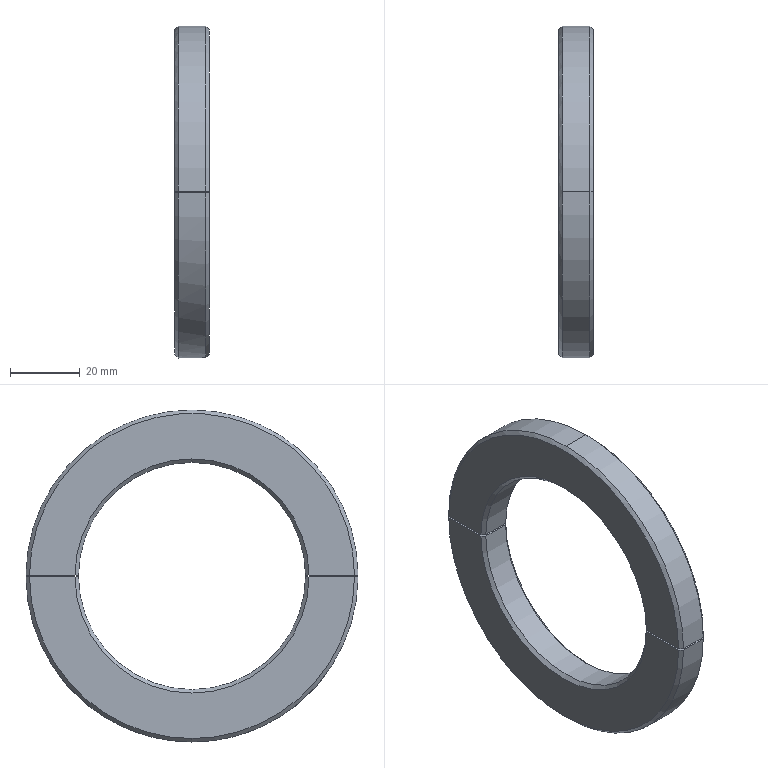Part | SolidWorks | features Chamfer 1, Extrusion 1, ICE 1 | 2 solids | 26 faces | box 10 x 94.999 x 95 mm | volume 37048 mm3 | cone 12 | plane 8 | cylinder 6 | commonest cylinder face diameters 65 x3 95 x3
STEP:
#1=CARTESIAN_POINT('',(10.,0.,46.5));
#2=VERTEX_POINT('',#1);
#3=CARTESIAN_POINT('',(10.,-46.499,0.25));
#4=VERTEX_POINT('',#3);
#5=CARTESIAN_POINT('',(10.,0.,0.));
#6=DIRECTION('',(1.,0.,0.));
#7=DIRECTION('',(0.,0.,-1.));
#8=AXIS2_PLACEMENT_3D('',#5,#6,#7);
#9=CIRCLE('',#8,46.5);
#10=EDGE_CURVE('',#2,#4,#9,.T.);
#11=ORIENTED_EDGE('',*,*,#10,.F.);
#12=CARTESIAN_POINT('',(9.,0.,47.5));
#13=VERTEX_POINT('',#12);
#14=CARTESIAN_POINT('',(10.,0.,46.5));
#15=DIRECTION('',(-0.7071,0.,0.7071));
#16=VECTOR('',#15,1000.);
#17=LINE('',#14,#16);
#18=EDGE_CURVE('',#2,#13,#17,.T.);
#19=ORIENTED_EDGE('',*,*,#18,.T.);
#20=CARTESIAN_POINT('',(9.,-47.499,0.25));
#21=VERTEX_POINT('',#20);
#22=CARTESIAN_POINT('',(9.,0.,0.));
#23=DIRECTION('',(-1.,0.,0.));
#24=DIRECTION('',(0.,0.,-1.));
#25=AXIS2_PLACEMENT_3D('',#22,#23,#24);
#26=CIRCLE('',#25,47.5);
#27=EDGE_CURVE('',#21,#13,#26,.T.);
#28=ORIENTED_EDGE('',*,*,#27,.F.);
#29=CARTESIAN_POINT('',(10.,-46.499,0.25));
#30=CARTESIAN_POINT('',(9.667,-46.833,0.25));
#31=CARTESIAN_POINT('',(9.333,-47.166,0.25));
#32=CARTESIAN_POINT('',(9.,-47.499,0.25));
#33=B_SPLINE_CURVE_WITH_KNOTS('',3,(#29,#30,#31,#32),.UNSPECIFIED.,.F.,.F.,(4,4),(0.1327,0.1342),.UNSPECIFIED.);
#34=EDGE_CURVE('',#4,#21,#33,.T.);
#35=ORIENTED_EDGE('',*,*,#34,.F.);
#36=EDGE_LOOP('',(#11,#19,#28,#35));
#37=FACE_OUTER_BOUND('',#36,.T.);
#38=CARTESIAN_POINT('',(10.,0.,0.));
#39=DIRECTION('',(-1.,0.,0.));
#40=DIRECTION('',(0.,0.,1.));
#41=AXIS2_PLACEMENT_3D('',#38,#39,#40);
#42=CONICAL_SURFACE('',#41,46.5,0.7854);
#43=ADVANCED_FACE('',(#37),#42,.T.);
#44=CARTESIAN_POINT('',(1.,0.,32.5));
#45=VERTEX_POINT('',#44);
#46=CARTESIAN_POINT('',(1.,32.499,0.25));
#47=VERTEX_POINT('',#46);
#48=CARTESIAN_POINT('',(1.,0.,0.));
#49=DIRECTION('',(-1.,0.,0.));
#50=DIRECTION('',(0.,0.,-1.));
#51=AXIS2_PLACEMENT_3D('',#48,#49,#50);
#52=CIRCLE('',#51,32.5);
#53=EDGE_CURVE('',#45,#47,#52,.T.);
#54=ORIENTED_EDGE('',*,*,#53,.F.);
#55=CARTESIAN_POINT('',(0.,0.,33.5));
#56=VERTEX_POINT('',#55);
#57=CARTESIAN_POINT('',(0.,0.,33.5));
#58=DIRECTION('',(-0.7071,0.,0.7071));
#59=VECTOR('',#58,1000.);
#60=LINE('',#57,#59);
#61=EDGE_CURVE('',#45,#56,#60,.T.);
#62=ORIENTED_EDGE('',*,*,#61,.T.);
#63=CARTESIAN_POINT('',(0.,33.499,0.25));
#64=VERTEX_POINT('',#63);
#65=CARTESIAN_POINT('',(0.,0.,0.));
#66=DIRECTION('',(1.,0.,0.));
#67=DIRECTION('',(0.,0.,-1.));
#68=AXIS2_PLACEMENT_3D('',#65,#66,#67);
#69=CIRCLE('',#68,33.5);
#70=EDGE_CURVE('',#64,#56,#69,.T.);
#71=ORIENTED_EDGE('',*,*,#70,.F.);
#72=CARTESIAN_POINT('',(1.,32.499,0.25));
#73=CARTESIAN_POINT('',(0.6667,32.832,0.25));
#74=CARTESIAN_POINT('',(0.3333,33.166,0.25));
#75=CARTESIAN_POINT('',(0.,33.499,0.25));
#76=B_SPLINE_CURVE_WITH_KNOTS('',3,(#72,#73,#74,#75),.UNSPECIFIED.,.F.,.F.,(4,4),(0.09304,0.09446),.UNSPECIFIED.);
#77=EDGE_CURVE('',#47,#64,#76,.T.);
#78=ORIENTED_EDGE('',*,*,#77,.F.);
#79=EDGE_LOOP('',(#54,#62,#71,#78));
#80=FACE_OUTER_BOUND('',#79,.T.);
#81=CARTESIAN_POINT('',(0.,0.,0.));
#82=DIRECTION('',(-1.,0.,0.));
#83=DIRECTION('',(0.,0.,1.));
#84=AXIS2_PLACEMENT_3D('',#81,#82,#83);
#85=CONICAL_SURFACE('',#84,33.5,0.7854);
#86=ADVANCED_FACE('',(#80),#85,.F.);
#87=CARTESIAN_POINT('',(9.,32.499,0.25));
#88=VERTEX_POINT('',#87);
#89=CARTESIAN_POINT('',(9.,0.,32.5));
#90=VERTEX_POINT('',#89);
#91=CARTESIAN_POINT('',(9.,0.,0.));
#92=DIRECTION('',(1.,0.,0.));
#93=DIRECTION('',(0.,0.,-1.));
#94=AXIS2_PLACEMENT_3D('',#91,#92,#93);
#95=CIRCLE('',#94,32.5);
#96=EDGE_CURVE('',#88,#90,#95,.T.);
#97=ORIENTED_EDGE('',*,*,#96,.T.);
#98=CARTESIAN_POINT('',(10.,0.,32.5));
#99=DIRECTION('',(-1.,0.,0.));
#100=VECTOR('',#99,1000.);
#101=LINE('',#98,#100);
#102=EDGE_CURVE('',#90,#45,#101,.T.);
#103=ORIENTED_EDGE('',*,*,#102,.T.);
#104=ORIENTED_EDGE('',*,*,#53,.T.);
#105=CARTESIAN_POINT('',(10.,32.499,0.25));
#106=DIRECTION('',(-1.,0.,0.));
#107=VECTOR('',#106,1000.);
#108=LINE('',#105,#107);
#109=EDGE_CURVE('',#88,#47,#108,.T.);
#110=ORIENTED_EDGE('',*,*,#109,.F.);
#111=EDGE_LOOP('',(#97,#103,#104,#110));
#112=FACE_OUTER_BOUND('',#111,.T.);
#113=CARTESIAN_POINT('',(10.,0.,0.));
#114=DIRECTION('',(-1.,0.,0.));
#115=DIRECTION('',(0.,0.,1.));
#116=AXIS2_PLACEMENT_3D('',#113,#114,#115);
#117=CYLINDRICAL_SURFACE('',#116,32.5);
#118=ADVANCED_FACE('',(#112),#117,.F.);
#119=ORIENTED_EDGE('',*,*,#27,.T.);
#120=CARTESIAN_POINT('',(1.,0.,47.5));
#121=VERTEX_POINT('',#120);
#122=CARTESIAN_POINT('',(10.,0.,47.5));
#123=DIRECTION('',(-1.,0.,0.));
#124=VECTOR('',#123,1000.);
#125=LINE('',#122,#124);
#126=EDGE_CURVE('',#13,#121,#125,.T.);
#127=ORIENTED_EDGE('',*,*,#126,.T.);
#128=CARTESIAN_POINT('',(1.,-47.499,0.25));
#129=VERTEX_POINT('',#128);
#130=CARTESIAN_POINT('',(1.,0.,0.));
#131=DIRECTION('',(1.,0.,0.));
#132=DIRECTION('',(0.,0.,-1.));
#133=AXIS2_PLACEMENT_3D('',#130,#131,#132);
#134=CIRCLE('',#133,47.5);
#135=EDGE_CURVE('',#121,#129,#134,.T.);
#136=ORIENTED_EDGE('',*,*,#135,.T.);
#137=CARTESIAN_POINT('',(10.,-47.499,0.25));
#138=DIRECTION('',(1.,0.,0.));
#139=VECTOR('',#138,1000.);
#140=LINE('',#137,#139);
#141=EDGE_CURVE('',#129,#21,#140,.T.);
#142=ORIENTED_EDGE('',*,*,#141,.T.);
#143=EDGE_LOOP('',(#119,#127,#136,#142));
#144=FACE_OUTER_BOUND('',#143,.T.);
#145=CARTESIAN_POINT('',(10.,0.,0.));
#146=DIRECTION('',(-1.,0.,0.));
#147=DIRECTION('',(0.,0.,1.));
#148=AXIS2_PLACEMENT_3D('',#145,#146,#147);
#149=CYLINDRICAL_SURFACE('',#148,47.5);
#150=ADVANCED_FACE('',(#144),#149,.T.);
#151=CARTESIAN_POINT('',(10.,33.499,0.25));
#152=VERTEX_POINT('',#151);
#153=CARTESIAN_POINT('',(10.,46.499,0.25));
#154=VERTEX_POINT('',#153);
#155=CARTESIAN_POINT('',(10.,79.674,0.25));
#156=DIRECTION('',(0.,1.,0.));
#157=VECTOR('',#156,1000.);
#158=LINE('',#155,#157);
#159=EDGE_CURVE('',#152,#154,#158,.T.);
#160=ORIENTED_EDGE('',*,*,#159,.T.);
#161=CARTESIAN_POINT('',(10.,0.,0.));
#162=DIRECTION('',(1.,0.,0.));
#163=DIRECTION('',(0.,0.,-1.));
#164=AXIS2_PLACEMENT_3D('',#161,#162,#163);
#165=CIRCLE('',#164,46.5);
#166=EDGE_CURVE('',#154,#2,#165,.T.);
#167=ORIENTED_EDGE('',*,*,#166,.T.);
#168=ORIENTED_EDGE('',*,*,#10,.T.);
#169=CARTESIAN_POINT('',(10.,-33.499,0.25));
#170=VERTEX_POINT('',#169);
#171=CARTESIAN_POINT('',(10.,79.674,0.25));
#172=DIRECTION('',(0.,1.,0.));
#173=VECTOR('',#172,1000.);
#174=LINE('',#171,#173);
#175=EDGE_CURVE('',#4,#170,#174,.T.);
#176=ORIENTED_EDGE('',*,*,#175,.T.);
#177=CARTESIAN_POINT('',(10.,0.,0.));
#178=DIRECTION('',(-1.,0.,0.));
#179=DIRECTION('',(0.,0.,-1.));
#180=AXIS2_PLACEMENT_3D('',#177,#178,#179);
#181=CIRCLE('',#180,33.5);
#182=EDGE_CURVE('',#170,#152,#181,.T.);
#183=ORIENTED_EDGE('',*,*,#182,.T.);
#184=EDGE_LOOP('',(#160,#167,#168,#176,#183));
#185=FACE_OUTER_BOUND('',#184,.T.);
#186=CARTESIAN_POINT('',(10.,0.,0.));
#187=DIRECTION('',(1.,0.,0.));
#188=DIRECTION('',(0.,0.,-1.));
#189=AXIS2_PLACEMENT_3D('',#186,#187,#188);
#190=PLANE('',#189);
#191=ADVANCED_FACE('',(#185),#190,.T.);
#192=CARTESIAN_POINT('',(0.,-46.499,0.25));
#193=VERTEX_POINT('',#192);
#194=CARTESIAN_POINT('',(0.,46.499,0.25));
#195=VERTEX_POINT('',#194);
#196=CARTESIAN_POINT('',(0.,0.,0.));
#197=DIRECTION('',(-1.,0.,0.));
#198=DIRECTION('',(0.,0.,-1.));
#199=AXIS2_PLACEMENT_3D('',#196,#197,#198);
#200=CIRCLE('',#199,46.5);
#201=EDGE_CURVE('',#193,#195,#200,.T.);
#202=ORIENTED_EDGE('',*,*,#201,.T.);
#203=CARTESIAN_POINT('',(0.,79.674,0.25));
#204=DIRECTION('',(0.,1.,0.));
#205=VECTOR('',#204,1000.);
#206=LINE('',#203,#205);
#207=EDGE_CURVE('',#64,#195,#206,.T.);
#208=ORIENTED_EDGE('',*,*,#207,.F.);
#209=ORIENTED_EDGE('',*,*,#70,.T.);
#210=CARTESIAN_POINT('',(0.,-33.499,0.25));
#211=VERTEX_POINT('',#210);
#212=CARTESIAN_POINT('',(0.,0.,0.));
#213=DIRECTION('',(1.,0.,0.));
#214=DIRECTION('',(0.,0.,-1.));
#215=AXIS2_PLACEMENT_3D('',#212,#213,#214);
#216=CIRCLE('',#215,33.5);
#217=EDGE_CURVE('',#56,#211,#216,.T.);
#218=ORIENTED_EDGE('',*,*,#217,.T.);
#219=CARTESIAN_POINT('',(0.,79.674,0.25));
#220=DIRECTION('',(0.,1.,0.));
#221=VECTOR('',#220,1000.);
#222=LINE('',#219,#221);
#223=EDGE_CURVE('',#193,#211,#222,.T.);
#224=ORIENTED_EDGE('',*,*,#223,.F.);
#225=EDGE_LOOP('',(#202,#208,#209,#218,#224));
#226=FACE_OUTER_BOUND('',#225,.T.);
#227=CARTESIAN_POINT('',(0.,0.,0.));
#228=DIRECTION('',(1.,0.,0.));
#229=DIRECTION('',(0.,0.,-1.));
#230=AXIS2_PLACEMENT_3D('',#227,#228,#229);
#231=PLANE('',#230);
#232=ADVANCED_FACE('',(#226),#231,.F.);
#233=ORIENTED_EDGE('',*,*,#126,.F.);
#234=CARTESIAN_POINT('',(9.,47.499,0.25));
#235=VERTEX_POINT('',#234);
#236=CARTESIAN_POINT('',(9.,0.,0.));
#237=DIRECTION('',(-1.,0.,0.));
#238=DIRECTION('',(0.,0.,-1.));
#239=AXIS2_PLACEMENT_3D('',#236,#237,#238);
#240=CIRCLE('',#239,47.5);
#241=EDGE_CURVE('',#13,#235,#240,.T.);
#242=ORIENTED_EDGE('',*,*,#241,.T.);
#243=CARTESIAN_POINT('',(1.,47.499,0.25));
#244=VERTEX_POINT('',#243);
#245=CARTESIAN_POINT('',(10.,47.499,0.25));
#246=DIRECTION('',(-1.,0.,0.));
#247=VECTOR('',#246,1000.);
#248=LINE('',#245,#247);
#249=EDGE_CURVE('',#235,#244,#248,.T.);
#250=ORIENTED_EDGE('',*,*,#249,.T.);
#251=CARTESIAN_POINT('',(1.,0.,0.));
#252=DIRECTION('',(1.,0.,0.));
#253=DIRECTION('',(0.,0.,-1.));
#254=AXIS2_PLACEMENT_3D('',#251,#252,#253);
#255=CIRCLE('',#254,47.5);
#256=EDGE_CURVE('',#244,#121,#255,.T.);
#257=ORIENTED_EDGE('',*,*,#256,.T.);
#258=EDGE_LOOP('',(#233,#242,#250,#257));
#259=FACE_OUTER_BOUND('',#258,.T.);
#260=CARTESIAN_POINT('',(10.,0.,0.));
#261=DIRECTION('',(-1.,0.,0.));
#262=DIRECTION('',(0.,0.,1.));
#263=AXIS2_PLACEMENT_3D('',#260,#261,#262);
#264=CYLINDRICAL_SURFACE('',#263,47.5);
#265=ADVANCED_FACE('',(#259),#264,.T.);
#266=ORIENTED_EDGE('',*,*,#102,.F.);
#267=CARTESIAN_POINT('',(9.,-32.499,0.25));
#268=VERTEX_POINT('',#267);
#269=CARTESIAN_POINT('',(9.,0.,0.));
#270=DIRECTION('',(1.,0.,0.));
#271=DIRECTION('',(0.,0.,-1.));
#272=AXIS2_PLACEMENT_3D('',#269,#270,#271);
#273=CIRCLE('',#272,32.5);
#274=EDGE_CURVE('',#90,#268,#273,.T.);
#275=ORIENTED_EDGE('',*,*,#274,.T.);
#276=CARTESIAN_POINT('',(1.,-32.499,0.25));
#277=VERTEX_POINT('',#276);
#278=CARTESIAN_POINT('',(10.,-32.499,0.25));
#279=DIRECTION('',(1.,0.,0.));
#280=VECTOR('',#279,1000.);
#281=LINE('',#278,#280);
#282=EDGE_CURVE('',#277,#268,#281,.T.);
#283=ORIENTED_EDGE('',*,*,#282,.F.);
#284=CARTESIAN_POINT('',(1.,0.,0.));
#285=DIRECTION('',(-1.,0.,0.));
#286=DIRECTION('',(0.,0.,-1.));
#287=AXIS2_PLACEMENT_3D('',#284,#285,#286);
#288=CIRCLE('',#287,32.5);
#289=EDGE_CURVE('',#277,#45,#288,.T.);
#290=ORIENTED_EDGE('',*,*,#289,.T.);
#291=EDGE_LOOP('',(#266,#275,#283,#290));
#292=FACE_OUTER_BOUND('',#291,.T.);
#293=CARTESIAN_POINT('',(10.,0.,0.));
#294=DIRECTION('',(-1.,0.,0.));
#295=DIRECTION('',(0.,0.,1.));
#296=AXIS2_PLACEMENT_3D('',#293,#294,#295);
#297=CYLINDRICAL_SURFACE('',#296,32.5);
#298=ADVANCED_FACE('',(#292),#297,.F.);
#299=ORIENTED_EDGE('',*,*,#61,.F.);
#300=ORIENTED_EDGE('',*,*,#289,.F.);
#301=CARTESIAN_POINT('',(0.,-33.499,0.25));
#302=CARTESIAN_POINT('',(0.3333,-33.166,0.25));
#303=CARTESIAN_POINT('',(0.6667,-32.832,0.25));
#304=CARTESIAN_POINT('',(1.,-32.499,0.25));
#305=B_SPLINE_CURVE_WITH_KNOTS('',3,(#301,#302,#303,#304),.UNSPECIFIED.,.F.,.F.,(4,4),(0.00000099,0.001415),.UNSPECIFIED.);
#306=EDGE_CURVE('',#211,#277,#305,.T.);
#307=ORIENTED_EDGE('',*,*,#306,.F.);
#308=ORIENTED_EDGE('',*,*,#217,.F.);
#309=EDGE_LOOP('',(#299,#300,#307,#308));
#310=FACE_OUTER_BOUND('',#309,.T.);
#311=CARTESIAN_POINT('',(0.,0.,0.));
#312=DIRECTION('',(-1.,0.,0.));
#313=DIRECTION('',(0.,0.,1.));
#314=AXIS2_PLACEMENT_3D('',#311,#312,#313);
#315=CONICAL_SURFACE('',#314,33.5,0.7854);
#316=ADVANCED_FACE('',(#310),#315,.F.);
#317=CARTESIAN_POINT('',(10.,33.499,0.25));
#318=CARTESIAN_POINT('',(9.667,33.166,0.25));
#319=CARTESIAN_POINT('',(9.333,32.832,0.25));
#320=CARTESIAN_POINT('',(9.,32.499,0.25));
#321=B_SPLINE_CURVE_WITH_KNOTS('',3,(#317,#318,#319,#320),.UNSPECIFIED.,.F.,.F.,(4,4),(0.00000099,0.001415),.UNSPECIFIED.);
#322=EDGE_CURVE('',#152,#88,#321,.T.);
#323=ORIENTED_EDGE('',*,*,#322,.F.);
#324=ORIENTED_EDGE('',*,*,#182,.F.);
#325=CARTESIAN_POINT('',(9.,-32.499,0.25));
#326=CARTESIAN_POINT('',(9.333,-32.832,0.25));
#327=CARTESIAN_POINT('',(9.667,-33.166,0.25));
#328=CARTESIAN_POINT('',(10.,-33.499,0.25));
#329=B_SPLINE_CURVE_WITH_KNOTS('',3,(#325,#326,#327,#328),.UNSPECIFIED.,.F.,.F.,(4,4),(0.09304,0.09446),.UNSPECIFIED.);
#330=EDGE_CURVE('',#268,#170,#329,.T.);
#331=ORIENTED_EDGE('',*,*,#330,.F.);
#332=ORIENTED_EDGE('',*,*,#274,.F.);
#333=ORIENTED_EDGE('',*,*,#96,.F.);
#334=EDGE_LOOP('',(#323,#324,#331,#332,#333));
#335=FACE_OUTER_BOUND('',#334,.T.);
#336=CARTESIAN_POINT('',(9.,0.,0.));
#337=DIRECTION('',(1.,0.,0.));
#338=DIRECTION('',(0.,0.,-1.));
#339=AXIS2_PLACEMENT_3D('',#336,#337,#338);
#340=CONICAL_SURFACE('',#339,32.5,0.7854);
#341=ADVANCED_FACE('',(#335),#340,.F.);
#342=CARTESIAN_POINT('',(1.,-47.499,0.25));
#343=CARTESIAN_POINT('',(0.6667,-47.166,0.25));
#344=CARTESIAN_POINT('',(0.3333,-46.833,0.25));
#345=CARTESIAN_POINT('',(0.,-46.499,0.25));
#346=B_SPLINE_CURVE_WITH_KNOTS('',3,(#342,#343,#344,#345),.UNSPECIFIED.,.F.,.F.,(4,4),(0.00000099,0.001415),.UNSPECIFIED.);
#347=EDGE_CURVE('',#129,#193,#346,.T.);
#348=ORIENTED_EDGE('',*,*,#347,.F.);
#349=ORIENTED_EDGE('',*,*,#135,.F.);
#350=ORIENTED_EDGE('',*,*,#256,.F.);
#351=CARTESIAN_POINT('',(0.,46.499,0.25));
#352=CARTESIAN_POINT('',(0.3333,46.833,0.25));
#353=CARTESIAN_POINT('',(0.6667,47.166,0.25));
#354=CARTESIAN_POINT('',(1.,47.499,0.25));
#355=B_SPLINE_CURVE_WITH_KNOTS('',3,(#351,#352,#353,#354),.UNSPECIFIED.,.F.,.F.,(4,4),(0.1327,0.1342),.UNSPECIFIED.);
#356=EDGE_CURVE('',#195,#244,#355,.T.);
#357=ORIENTED_EDGE('',*,*,#356,.F.);
#358=ORIENTED_EDGE('',*,*,#201,.F.);
#359=EDGE_LOOP('',(#348,#349,#350,#357,#358));
#360=FACE_OUTER_BOUND('',#359,.T.);
#361=CARTESIAN_POINT('',(1.,0.,0.));
#362=DIRECTION('',(1.,0.,0.));
#363=DIRECTION('',(0.,0.,-1.));
#364=AXIS2_PLACEMENT_3D('',#361,#362,#363);
#365=CONICAL_SURFACE('',#364,47.5,0.7854);
#366=ADVANCED_FACE('',(#360),#365,.T.);
#367=ORIENTED_EDGE('',*,*,#18,.F.);
#368=ORIENTED_EDGE('',*,*,#166,.F.);
#369=CARTESIAN_POINT('',(9.,47.499,0.25));
#370=CARTESIAN_POINT('',(9.333,47.166,0.25));
#371=CARTESIAN_POINT('',(9.667,46.833,0.25));
#372=CARTESIAN_POINT('',(10.,46.499,0.25));
#373=B_SPLINE_CURVE_WITH_KNOTS('',3,(#369,#370,#371,#372),.UNSPECIFIED.,.F.,.F.,(4,4),(0.00000099,0.001415),.UNSPECIFIED.);
#374=EDGE_CURVE('',#235,#154,#373,.T.);
#375=ORIENTED_EDGE('',*,*,#374,.F.);
#376=ORIENTED_EDGE('',*,*,#241,.F.);
#377=EDGE_LOOP('',(#367,#368,#375,#376));
#378=FACE_OUTER_BOUND('',#377,.T.);
#379=CARTESIAN_POINT('',(10.,0.,0.));
#380=DIRECTION('',(-1.,0.,0.));
#381=DIRECTION('',(0.,0.,1.));
#382=AXIS2_PLACEMENT_3D('',#379,#380,#381);
#383=CONICAL_SURFACE('',#382,46.5,0.7854);
#384=ADVANCED_FACE('',(#378),#383,.T.);
#385=ORIENTED_EDGE('',*,*,#306,.T.);
#386=ORIENTED_EDGE('',*,*,#282,.T.);
#387=ORIENTED_EDGE('',*,*,#330,.T.);
#388=ORIENTED_EDGE('',*,*,#175,.F.);
#389=ORIENTED_EDGE('',*,*,#34,.T.);
#390=ORIENTED_EDGE('',*,*,#141,.F.);
#391=ORIENTED_EDGE('',*,*,#347,.T.);
#392=ORIENTED_EDGE('',*,*,#223,.T.);
#393=EDGE_LOOP('',(#385,#386,#387,#388,#389,#390,#391,#392));
#394=FACE_OUTER_BOUND('',#393,.T.);
#395=CARTESIAN_POINT('',(10.,79.674,0.25));
#396=DIRECTION('',(0.,0.,1.));
#397=DIRECTION('',(0.,-1.,0.));
#398=AXIS2_PLACEMENT_3D('',#395,#396,#397);
#399=PLANE('',#398);
#400=ADVANCED_FACE('',(#394),#399,.F.);
#401=ORIENTED_EDGE('',*,*,#77,.T.);
#402=ORIENTED_EDGE('',*,*,#207,.T.);
#403=ORIENTED_EDGE('',*,*,#356,.T.);
#404=ORIENTED_EDGE('',*,*,#249,.F.);
#405=ORIENTED_EDGE('',*,*,#374,.T.);
#406=ORIENTED_EDGE('',*,*,#159,.F.);
#407=ORIENTED_EDGE('',*,*,#322,.T.);
#408=ORIENTED_EDGE('',*,*,#109,.T.);
#409=EDGE_LOOP('',(#401,#402,#403,#404,#405,#406,#407,#408));
#410=FACE_OUTER_BOUND('',#409,.T.);
#411=CARTESIAN_POINT('',(10.,79.674,0.25));
#412=DIRECTION('',(0.,0.,1.));
#413=DIRECTION('',(0.,-1.,0.));
#414=AXIS2_PLACEMENT_3D('',#411,#412,#413);
#415=PLANE('',#414);
#416=ADVANCED_FACE('',(#410),#415,.F.);
#417=CLOSED_SHELL('',(#43,#86,#118,#150,#191,#232,#265,#298,#316,#341,#366,#384,#400,#416));
#418=MANIFOLD_SOLID_BREP('',#417);
#419=CARTESIAN_POINT('',(0.,0.,-46.5));
#420=VERTEX_POINT('',#419);
#421=CARTESIAN_POINT('',(0.,-46.499,-0.25));
#422=VERTEX_POINT('',#421);
#423=CARTESIAN_POINT('',(0.,0.,0.));
#424=DIRECTION('',(-1.,0.,0.));
#425=DIRECTION('',(0.,0.,-1.));
#426=AXIS2_PLACEMENT_3D('',#423,#424,#425);
#427=CIRCLE('',#426,46.5);
#428=EDGE_CURVE('',#420,#422,#427,.T.);
#429=ORIENTED_EDGE('',*,*,#428,.F.);
#430=CARTESIAN_POINT('',(1.,0.,-47.5));
#431=VERTEX_POINT('',#430);
#432=CARTESIAN_POINT('',(1.,0.,-47.5));
#433=DIRECTION('',(0.7071,0.,-0.7071));
#434=VECTOR('',#433,1000.);
#435=LINE('',#432,#434);
#436=EDGE_CURVE('',#420,#431,#435,.T.);
#437=ORIENTED_EDGE('',*,*,#436,.T.);
#438=CARTESIAN_POINT('',(1.,-47.499,-0.25));
#439=VERTEX_POINT('',#438);
#440=CARTESIAN_POINT('',(1.,0.,0.));
#441=DIRECTION('',(1.,0.,0.));
#442=DIRECTION('',(0.,0.,-1.));
#443=AXIS2_PLACEMENT_3D('',#440,#441,#442);
#444=CIRCLE('',#443,47.5);
#445=EDGE_CURVE('',#439,#431,#444,.T.);
#446=ORIENTED_EDGE('',*,*,#445,.F.);
#447=CARTESIAN_POINT('',(0.,-46.499,-0.25));
#448=CARTESIAN_POINT('',(0.3333,-46.833,-0.25));
#449=CARTESIAN_POINT('',(0.6667,-47.166,-0.25));
#450=CARTESIAN_POINT('',(1.,-47.499,-0.25));
#451=B_SPLINE_CURVE_WITH_KNOTS('',3,(#447,#448,#449,#450),.UNSPECIFIED.,.F.,.F.,(4,4),(0.1327,0.1342),.UNSPECIFIED.);
#452=EDGE_CURVE('',#422,#439,#451,.T.);
#453=ORIENTED_EDGE('',*,*,#452,.F.);
#454=EDGE_LOOP('',(#429,#437,#446,#453));
#455=FACE_OUTER_BOUND('',#454,.T.);
#456=CARTESIAN_POINT('',(1.,0.,0.));
#457=DIRECTION('',(1.,0.,0.));
#458=DIRECTION('',(0.,0.,-1.));
#459=AXIS2_PLACEMENT_3D('',#456,#457,#458);
#460=CONICAL_SURFACE('',#459,47.5,0.7854);
#461=ADVANCED_FACE('',(#455),#460,.T.);
#462=CARTESIAN_POINT('',(9.,0.,-32.5));
#463=VERTEX_POINT('',#462);
#464=CARTESIAN_POINT('',(9.,32.499,-0.25));
#465=VERTEX_POINT('',#464);
#466=CARTESIAN_POINT('',(9.,0.,0.));
#467=DIRECTION('',(1.,0.,0.));
#468=DIRECTION('',(0.,0.,-1.));
#469=AXIS2_PLACEMENT_3D('',#466,#467,#468);
#470=CIRCLE('',#469,32.5);
#471=EDGE_CURVE('',#463,#465,#470,.T.);
#472=ORIENTED_EDGE('',*,*,#471,.F.);
#473=CARTESIAN_POINT('',(10.,0.,-33.5));
#474=VERTEX_POINT('',#473);
#475=CARTESIAN_POINT('',(9.,0.,-32.5));
#476=DIRECTION('',(0.7071,0.,-0.7071));
#477=VECTOR('',#476,1000.);
#478=LINE('',#475,#477);
#479=EDGE_CURVE('',#463,#474,#478,.T.);
#480=ORIENTED_EDGE('',*,*,#479,.T.);
#481=CARTESIAN_POINT('',(10.,33.499,-0.25));
#482=VERTEX_POINT('',#481);
#483=CARTESIAN_POINT('',(10.,0.,0.));
#484=DIRECTION('',(-1.,0.,0.));
#485=DIRECTION('',(0.,0.,-1.));
#486=AXIS2_PLACEMENT_3D('',#483,#484,#485);
#487=CIRCLE('',#486,33.5);
#488=EDGE_CURVE('',#482,#474,#487,.T.);
#489=ORIENTED_EDGE('',*,*,#488,.F.);
#490=CARTESIAN_POINT('',(9.,32.499,-0.25));
#491=CARTESIAN_POINT('',(9.333,32.832,-0.25));
#492=CARTESIAN_POINT('',(9.667,33.166,-0.25));
#493=CARTESIAN_POINT('',(10.,33.499,-0.25));
#494=B_SPLINE_CURVE_WITH_KNOTS('',3,(#490,#491,#492,#493),.UNSPECIFIED.,.F.,.F.,(4,4),(0.09304,0.09446),.UNSPECIFIED.);
#495=EDGE_CURVE('',#465,#482,#494,.T.);
#496=ORIENTED_EDGE('',*,*,#495,.F.);
#497=EDGE_LOOP('',(#472,#480,#489,#496));
#498=FACE_OUTER_BOUND('',#497,.T.);
#499=CARTESIAN_POINT('',(9.,0.,0.));
#500=DIRECTION('',(1.,0.,0.));
#501=DIRECTION('',(0.,0.,-1.));
#502=AXIS2_PLACEMENT_3D('',#499,#500,#501);
#503=CONICAL_SURFACE('',#502,32.5,0.7854);
#504=ADVANCED_FACE('',(#498),#503,.F.);
#505=CARTESIAN_POINT('',(0.,33.499,-0.25));
#506=VERTEX_POINT('',#505);
#507=CARTESIAN_POINT('',(1.,32.499,-0.25));
#508=VERTEX_POINT('',#507);
#509=CARTESIAN_POINT('',(0.,33.499,-0.25));
#510=CARTESIAN_POINT('',(0.3333,33.166,-0.25));
#511=CARTESIAN_POINT('',(0.6667,32.832,-0.25));
#512=CARTESIAN_POINT('',(1.,32.499,-0.25));
#513=B_SPLINE_CURVE_WITH_KNOTS('',3,(#509,#510,#511,#512),.UNSPECIFIED.,.F.,.F.,(4,4),(0.00000099,0.001415),.UNSPECIFIED.);
#514=EDGE_CURVE('',#506,#508,#513,.T.);
#515=ORIENTED_EDGE('',*,*,#514,.F.);
#516=CARTESIAN_POINT('',(0.,-33.499,-0.25));
#517=VERTEX_POINT('',#516);
#518=CARTESIAN_POINT('',(0.,0.,0.));
#519=DIRECTION('',(1.,0.,0.));
#520=DIRECTION('',(0.,0.,-1.));
#521=AXIS2_PLACEMENT_3D('',#518,#519,#520);
#522=CIRCLE('',#521,33.5);
#523=EDGE_CURVE('',#517,#506,#522,.T.);
#524=ORIENTED_EDGE('',*,*,#523,.F.);
#525=CARTESIAN_POINT('',(1.,-32.499,-0.25));
#526=VERTEX_POINT('',#525);
#527=CARTESIAN_POINT('',(1.,-32.499,-0.25));
#528=CARTESIAN_POINT('',(0.6667,-32.832,-0.25));
#529=CARTESIAN_POINT('',(0.3333,-33.166,-0.25));
#530=CARTESIAN_POINT('',(0.,-33.499,-0.25));
#531=B_SPLINE_CURVE_WITH_KNOTS('',3,(#527,#528,#529,#530),.UNSPECIFIED.,.F.,.F.,(4,4),(0.09304,0.09446),.UNSPECIFIED.);
#532=EDGE_CURVE('',#526,#517,#531,.T.);
#533=ORIENTED_EDGE('',*,*,#532,.F.);
#534=CARTESIAN_POINT('',(1.,0.,0.));
#535=DIRECTION('',(-1.,0.,0.));
#536=DIRECTION('',(0.,0.,-1.));
#537=AXIS2_PLACEMENT_3D('',#534,#535,#536);
#538=CIRCLE('',#537,32.5);
#539=EDGE_CURVE('',#508,#526,#538,.T.);
#540=ORIENTED_EDGE('',*,*,#539,.F.);
#541=EDGE_LOOP('',(#515,#524,#533,#540));
#542=FACE_OUTER_BOUND('',#541,.T.);
#543=CARTESIAN_POINT('',(0.,0.,0.));
#544=DIRECTION('',(-1.,0.,0.));
#545=DIRECTION('',(0.,0.,1.));
#546=AXIS2_PLACEMENT_3D('',#543,#544,#545);
#547=CONICAL_SURFACE('',#546,33.5,0.7854);
#548=ADVANCED_FACE('',(#542),#547,.F.);
#549=ORIENTED_EDGE('',*,*,#479,.F.);
#550=CARTESIAN_POINT('',(9.,-32.499,-0.25));
#551=VERTEX_POINT('',#550);
#552=CARTESIAN_POINT('',(9.,0.,0.));
#553=DIRECTION('',(1.,0.,0.));
#554=DIRECTION('',(0.,0.,-1.));
#555=AXIS2_PLACEMENT_3D('',#552,#553,#554);
#556=CIRCLE('',#555,32.5);
#557=EDGE_CURVE('',#551,#463,#556,.T.);
#558=ORIENTED_EDGE('',*,*,#557,.F.);
#559=CARTESIAN_POINT('',(10.,-33.499,-0.25));
#560=VERTEX_POINT('',#559);
#561=CARTESIAN_POINT('',(10.,-33.499,-0.25));
#562=CARTESIAN_POINT('',(9.667,-33.166,-0.25));
#563=CARTESIAN_POINT('',(9.333,-32.832,-0.25));
#564=CARTESIAN_POINT('',(9.,-32.499,-0.25));
#565=B_SPLINE_CURVE_WITH_KNOTS('',3,(#561,#562,#563,#564),.UNSPECIFIED.,.F.,.F.,(4,4),(0.00000099,0.001415),.UNSPECIFIED.);
#566=EDGE_CURVE('',#560,#551,#565,.T.);
#567=ORIENTED_EDGE('',*,*,#566,.F.);
#568=CARTESIAN_POINT('',(10.,0.,0.));
#569=DIRECTION('',(-1.,0.,0.));
#570=DIRECTION('',(0.,0.,-1.));
#571=AXIS2_PLACEMENT_3D('',#568,#569,#570);
#572=CIRCLE('',#571,33.5);
#573=EDGE_CURVE('',#474,#560,#572,.T.);
#574=ORIENTED_EDGE('',*,*,#573,.F.);
#575=EDGE_LOOP('',(#549,#558,#567,#574));
#576=FACE_OUTER_BOUND('',#575,.T.);
#577=CARTESIAN_POINT('',(9.,0.,0.));
#578=DIRECTION('',(1.,0.,0.));
#579=DIRECTION('',(0.,0.,-1.));
#580=AXIS2_PLACEMENT_3D('',#577,#578,#579);
#581=CONICAL_SURFACE('',#580,32.5,0.7854);
#582=ADVANCED_FACE('',(#576),#581,.F.);
#583=CARTESIAN_POINT('',(10.,-32.499,-0.25));
#584=DIRECTION('',(-1.,0.,0.));
#585=VECTOR('',#584,1000.);
#586=LINE('',#583,#585);
#587=EDGE_CURVE('',#551,#526,#586,.T.);
#588=ORIENTED_EDGE('',*,*,#587,.F.);
#589=ORIENTED_EDGE('',*,*,#557,.T.);
#590=ORIENTED_EDGE('',*,*,#471,.T.);
#591=CARTESIAN_POINT('',(10.,32.499,-0.25));
#592=DIRECTION('',(1.,0.,0.));
#593=VECTOR('',#592,1000.);
#594=LINE('',#591,#593);
#595=EDGE_CURVE('',#508,#465,#594,.T.);
#596=ORIENTED_EDGE('',*,*,#595,.F.);
#597=ORIENTED_EDGE('',*,*,#539,.T.);
#598=EDGE_LOOP('',(#588,#589,#590,#596,#597));
#599=FACE_OUTER_BOUND('',#598,.T.);
#600=CARTESIAN_POINT('',(10.,0.,0.));
#601=DIRECTION('',(-1.,0.,0.));
#602=DIRECTION('',(0.,0.,1.));
#603=AXIS2_PLACEMENT_3D('',#600,#601,#602);
#604=CYLINDRICAL_SURFACE('',#603,32.5);
#605=ADVANCED_FACE('',(#599),#604,.F.);
#606=ORIENTED_EDGE('',*,*,#436,.F.);
#607=CARTESIAN_POINT('',(0.,46.499,-0.25));
#608=VERTEX_POINT('',#607);
#609=CARTESIAN_POINT('',(0.,0.,0.));
#610=DIRECTION('',(-1.,0.,0.));
#611=DIRECTION('',(0.,0.,-1.));
#612=AXIS2_PLACEMENT_3D('',#609,#610,#611);
#613=CIRCLE('',#612,46.5);
#614=EDGE_CURVE('',#608,#420,#613,.T.);
#615=ORIENTED_EDGE('',*,*,#614,.F.);
#616=CARTESIAN_POINT('',(1.,47.499,-0.25));
#617=VERTEX_POINT('',#616);
#618=CARTESIAN_POINT('',(1.,47.499,-0.25));
#619=CARTESIAN_POINT('',(0.6667,47.166,-0.25));
#620=CARTESIAN_POINT('',(0.3333,46.833,-0.25));
#621=CARTESIAN_POINT('',(0.,46.499,-0.25));
#622=B_SPLINE_CURVE_WITH_KNOTS('',3,(#618,#619,#620,#621),.UNSPECIFIED.,.F.,.F.,(4,4),(0.00000099,0.001415),.UNSPECIFIED.);
#623=EDGE_CURVE('',#617,#608,#622,.T.);
#624=ORIENTED_EDGE('',*,*,#623,.F.);
#625=CARTESIAN_POINT('',(1.,0.,0.));
#626=DIRECTION('',(1.,0.,0.));
#627=DIRECTION('',(0.,0.,-1.));
#628=AXIS2_PLACEMENT_3D('',#625,#626,#627);
#629=CIRCLE('',#628,47.5);
#630=EDGE_CURVE('',#431,#617,#629,.T.);
#631=ORIENTED_EDGE('',*,*,#630,.F.);
#632=EDGE_LOOP('',(#606,#615,#624,#631));
#633=FACE_OUTER_BOUND('',#632,.T.);
#634=CARTESIAN_POINT('',(1.,0.,0.));
#635=DIRECTION('',(1.,0.,0.));
#636=DIRECTION('',(0.,0.,-1.));
#637=AXIS2_PLACEMENT_3D('',#634,#635,#636);
#638=CONICAL_SURFACE('',#637,47.5,0.7854);
#639=ADVANCED_FACE('',(#633),#638,.T.);
#640=CARTESIAN_POINT('',(9.,-47.499,-0.25));
#641=VERTEX_POINT('',#640);
#642=CARTESIAN_POINT('',(10.,-46.499,-0.25));
#643=VERTEX_POINT('',#642);
#644=CARTESIAN_POINT('',(9.,-47.499,-0.25));
#645=CARTESIAN_POINT('',(9.333,-47.166,-0.25));
#646=CARTESIAN_POINT('',(9.667,-46.833,-0.25));
#647=CARTESIAN_POINT('',(10.,-46.499,-0.25));
#648=B_SPLINE_CURVE_WITH_KNOTS('',3,(#644,#645,#646,#647),.UNSPECIFIED.,.F.,.F.,(4,4),(0.00000099,0.001415),.UNSPECIFIED.);
#649=EDGE_CURVE('',#641,#643,#648,.T.);
#650=ORIENTED_EDGE('',*,*,#649,.F.);
#651=CARTESIAN_POINT('',(9.,47.499,-0.25));
#652=VERTEX_POINT('',#651);
#653=CARTESIAN_POINT('',(9.,0.,0.));
#654=DIRECTION('',(-1.,0.,0.));
#655=DIRECTION('',(0.,0.,-1.));
#656=AXIS2_PLACEMENT_3D('',#653,#654,#655);
#657=CIRCLE('',#656,47.5);
#658=EDGE_CURVE('',#652,#641,#657,.T.);
#659=ORIENTED_EDGE('',*,*,#658,.F.);
#660=CARTESIAN_POINT('',(10.,46.499,-0.25));
#661=VERTEX_POINT('',#660);
#662=CARTESIAN_POINT('',(10.,46.499,-0.25));
#663=CARTESIAN_POINT('',(9.667,46.833,-0.25));
#664=CARTESIAN_POINT('',(9.333,47.166,-0.25));
#665=CARTESIAN_POINT('',(9.,47.499,-0.25));
#666=B_SPLINE_CURVE_WITH_KNOTS('',3,(#662,#663,#664,#665),.UNSPECIFIED.,.F.,.F.,(4,4),(0.1327,0.1342),.UNSPECIFIED.);
#667=EDGE_CURVE('',#661,#652,#666,.T.);
#668=ORIENTED_EDGE('',*,*,#667,.F.);
#669=CARTESIAN_POINT('',(10.,0.,0.));
#670=DIRECTION('',(1.,0.,0.));
#671=DIRECTION('',(0.,0.,-1.));
#672=AXIS2_PLACEMENT_3D('',#669,#670,#671);
#673=CIRCLE('',#672,46.5);
#674=EDGE_CURVE('',#643,#661,#673,.T.);
#675=ORIENTED_EDGE('',*,*,#674,.F.);
#676=EDGE_LOOP('',(#650,#659,#668,#675));
#677=FACE_OUTER_BOUND('',#676,.T.);
#678=CARTESIAN_POINT('',(10.,0.,0.));
#679=DIRECTION('',(-1.,0.,0.));
#680=DIRECTION('',(0.,0.,1.));
#681=AXIS2_PLACEMENT_3D('',#678,#679,#680);
#682=CONICAL_SURFACE('',#681,46.5,0.7854);
#683=ADVANCED_FACE('',(#677),#682,.T.);
#684=ORIENTED_EDGE('',*,*,#658,.T.);
#685=CARTESIAN_POINT('',(10.,-47.499,-0.25));
#686=DIRECTION('',(-1.,0.,0.));
#687=VECTOR('',#686,1000.);
#688=LINE('',#685,#687);
#689=EDGE_CURVE('',#641,#439,#688,.T.);
#690=ORIENTED_EDGE('',*,*,#689,.T.);
#691=ORIENTED_EDGE('',*,*,#445,.T.);
#692=ORIENTED_EDGE('',*,*,#630,.T.);
#693=CARTESIAN_POINT('',(10.,47.499,-0.25));
#694=DIRECTION('',(1.,0.,0.));
#695=VECTOR('',#694,1000.);
#696=LINE('',#693,#695);
#697=EDGE_CURVE('',#617,#652,#696,.T.);
#698=ORIENTED_EDGE('',*,*,#697,.T.);
#699=EDGE_LOOP('',(#684,#690,#691,#692,#698));
#700=FACE_OUTER_BOUND('',#699,.T.);
#701=CARTESIAN_POINT('',(10.,0.,0.));
#702=DIRECTION('',(-1.,0.,0.));
#703=DIRECTION('',(0.,0.,1.));
#704=AXIS2_PLACEMENT_3D('',#701,#702,#703);
#705=CYLINDRICAL_SURFACE('',#704,47.5);
#706=ADVANCED_FACE('',(#700),#705,.T.);
#707=ORIENTED_EDGE('',*,*,#614,.T.);
#708=ORIENTED_EDGE('',*,*,#428,.T.);
#709=CARTESIAN_POINT('',(0.,79.674,-0.25));
#710=DIRECTION('',(0.,-1.,0.));
#711=VECTOR('',#710,1000.);
#712=LINE('',#709,#711);
#713=EDGE_CURVE('',#517,#422,#712,.T.);
#714=ORIENTED_EDGE('',*,*,#713,.F.);
#715=ORIENTED_EDGE('',*,*,#523,.T.);
#716=CARTESIAN_POINT('',(0.,79.674,-0.25));
#717=DIRECTION('',(0.,-1.,0.));
#718=VECTOR('',#717,1000.);
#719=LINE('',#716,#718);
#720=EDGE_CURVE('',#608,#506,#719,.T.);
#721=ORIENTED_EDGE('',*,*,#720,.F.);
#722=EDGE_LOOP('',(#707,#708,#714,#715,#721));
#723=FACE_OUTER_BOUND('',#722,.T.);
#724=CARTESIAN_POINT('',(0.,0.,0.));
#725=DIRECTION('',(1.,0.,0.));
#726=DIRECTION('',(0.,0.,-1.));
#727=AXIS2_PLACEMENT_3D('',#724,#725,#726);
#728=PLANE('',#727);
#729=ADVANCED_FACE('',(#723),#728,.F.);
#730=CARTESIAN_POINT('',(10.,79.674,-0.25));
#731=DIRECTION('',(0.,-1.,0.));
#732=VECTOR('',#731,1000.);
#733=LINE('',#730,#732);
#734=EDGE_CURVE('',#560,#643,#733,.T.);
#735=ORIENTED_EDGE('',*,*,#734,.T.);
#736=ORIENTED_EDGE('',*,*,#674,.T.);
#737=CARTESIAN_POINT('',(10.,79.674,-0.25));
#738=DIRECTION('',(0.,-1.,0.));
#739=VECTOR('',#738,1000.);
#740=LINE('',#737,#739);
#741=EDGE_CURVE('',#661,#482,#740,.T.);
#742=ORIENTED_EDGE('',*,*,#741,.T.);
#743=ORIENTED_EDGE('',*,*,#488,.T.);
#744=ORIENTED_EDGE('',*,*,#573,.T.);
#745=EDGE_LOOP('',(#735,#736,#742,#743,#744));
#746=FACE_OUTER_BOUND('',#745,.T.);
#747=CARTESIAN_POINT('',(10.,0.,0.));
#748=DIRECTION('',(1.,0.,0.));
#749=DIRECTION('',(0.,0.,-1.));
#750=AXIS2_PLACEMENT_3D('',#747,#748,#749);
#751=PLANE('',#750);
#752=ADVANCED_FACE('',(#746),#751,.T.);
#753=ORIENTED_EDGE('',*,*,#514,.T.);
#754=ORIENTED_EDGE('',*,*,#595,.T.);
#755=ORIENTED_EDGE('',*,*,#495,.T.);
#756=ORIENTED_EDGE('',*,*,#741,.F.);
#757=ORIENTED_EDGE('',*,*,#667,.T.);
#758=ORIENTED_EDGE('',*,*,#697,.F.);
#759=ORIENTED_EDGE('',*,*,#623,.T.);
#760=ORIENTED_EDGE('',*,*,#720,.T.);
#761=EDGE_LOOP('',(#753,#754,#755,#756,#757,#758,#759,#760));
#762=FACE_OUTER_BOUND('',#761,.T.);
#763=CARTESIAN_POINT('',(10.,79.674,-0.25));
#764=DIRECTION('',(0.,0.,-1.));
#765=DIRECTION('',(0.,1.,0.));
#766=AXIS2_PLACEMENT_3D('',#763,#764,#765);
#767=PLANE('',#766);
#768=ADVANCED_FACE('',(#762),#767,.F.);
#769=ORIENTED_EDGE('',*,*,#532,.T.);
#770=ORIENTED_EDGE('',*,*,#713,.T.);
#771=ORIENTED_EDGE('',*,*,#452,.T.);
#772=ORIENTED_EDGE('',*,*,#689,.F.);
#773=ORIENTED_EDGE('',*,*,#649,.T.);
#774=ORIENTED_EDGE('',*,*,#734,.F.);
#775=ORIENTED_EDGE('',*,*,#566,.T.);
#776=ORIENTED_EDGE('',*,*,#587,.T.);
#777=EDGE_LOOP('',(#769,#770,#771,#772,#773,#774,#775,#776));
#778=FACE_OUTER_BOUND('',#777,.T.);
#779=CARTESIAN_POINT('',(10.,79.674,-0.25));
#780=DIRECTION('',(0.,0.,-1.));
#781=DIRECTION('',(0.,1.,0.));
#782=AXIS2_PLACEMENT_3D('',#779,#780,#781);
#783=PLANE('',#782);
#784=ADVANCED_FACE('',(#778),#783,.F.);
#785=CLOSED_SHELL('',(#461,#504,#548,#582,#605,#639,#683,#706,#729,#752,#768,#784));
#786=MANIFOLD_SOLID_BREP('',#785);
#787=CARTESIAN_POINT('',(0.,0.,0.));
#788=DIRECTION('',(0.,0.,1.));
#789=DIRECTION('',(1.,0.,0.));
#790=AXIS2_PLACEMENT_3D('',#787,#788,#789);
#791=(LENGTH_UNIT()NAMED_UNIT(*)SI_UNIT(.MILLI.,.METRE.));
#792=UNCERTAINTY_MEASURE_WITH_UNIT(LENGTH_MEASURE(0.00001),#791,'','');
#793=(NAMED_UNIT(*)PLANE_ANGLE_UNIT()SI_UNIT($,.RADIAN.));
#794=(NAMED_UNIT(*)SI_UNIT($,.STERADIAN.)SOLID_ANGLE_UNIT());
#795=(GEOMETRIC_REPRESENTATION_CONTEXT(3)GLOBAL_UNCERTAINTY_ASSIGNED_CONTEXT((#792))GLOBAL_UNIT_ASSIGNED_CONTEXT((#791,#793,#794))REPRESENTATION_CONTEXT('',''));
#796=ADVANCED_BREP_SHAPE_REPRESENTATION('',(#418,#786,#790),#795);